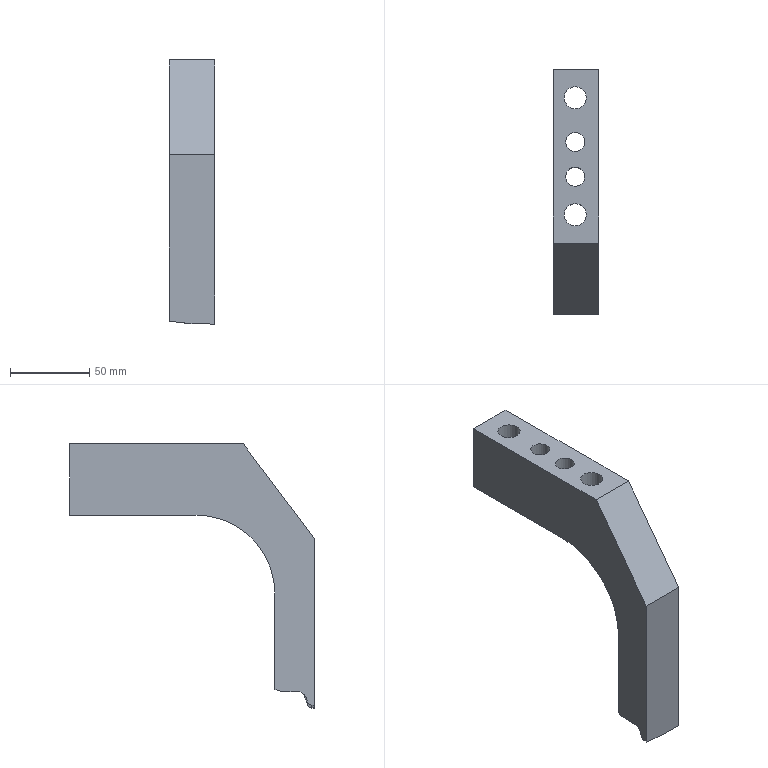Part | NX | features solid 2 | 1 solid | 31 faces | box 29 x 155 x 167.135 mm | volume 229983 mm3 | spline 16 | plane 8 | cylinder 7 | commonest cylinder face diameters 12 x2 14 x2 20 x2 100 x1